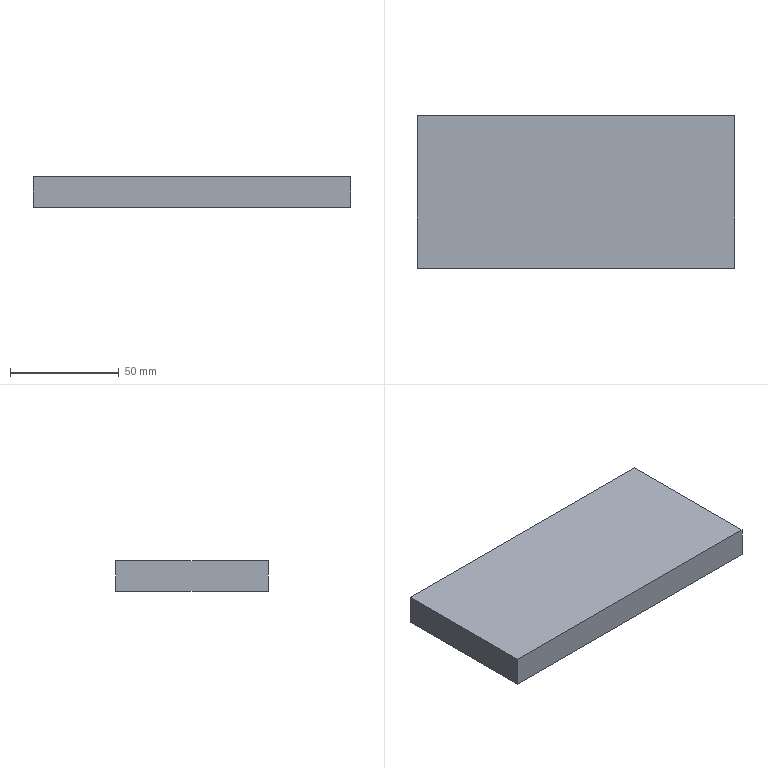Part | SolidWorks | features BaseBody 1 | 1 solid | 6 faces | box 146 x 70 x 14 mm | volume 143080 mm3 | plane 6
STEP:
#1=CARTESIAN_POINT('',(73.,-35.,-7.));
#2=VERTEX_POINT('',#1);
#3=CARTESIAN_POINT('',(73.,35.,-7.));
#4=VERTEX_POINT('',#3);
#5=CARTESIAN_POINT('',(73.,35.,-7.));
#6=DIRECTION('',(0.,1.,0.));
#7=VECTOR('',#6,1000.);
#8=LINE('',#5,#7);
#9=EDGE_CURVE('',#2,#4,#8,.T.);
#10=ORIENTED_EDGE('',*,*,#9,.T.);
#11=CARTESIAN_POINT('',(73.,35.,7.));
#12=VERTEX_POINT('',#11);
#13=CARTESIAN_POINT('',(73.,35.,7.));
#14=DIRECTION('',(0.,0.,-1.));
#15=VECTOR('',#14,1000.);
#16=LINE('',#13,#15);
#17=EDGE_CURVE('',#12,#4,#16,.T.);
#18=ORIENTED_EDGE('',*,*,#17,.F.);
#19=CARTESIAN_POINT('',(73.,-35.,7.));
#20=VERTEX_POINT('',#19);
#21=CARTESIAN_POINT('',(73.,35.,7.));
#22=DIRECTION('',(0.,1.,0.));
#23=VECTOR('',#22,1000.);
#24=LINE('',#21,#23);
#25=EDGE_CURVE('',#20,#12,#24,.T.);
#26=ORIENTED_EDGE('',*,*,#25,.F.);
#27=CARTESIAN_POINT('',(73.,-35.,7.));
#28=DIRECTION('',(0.,0.,-1.));
#29=VECTOR('',#28,1000.);
#30=LINE('',#27,#29);
#31=EDGE_CURVE('',#20,#2,#30,.T.);
#32=ORIENTED_EDGE('',*,*,#31,.T.);
#33=EDGE_LOOP('',(#10,#18,#26,#32));
#34=FACE_OUTER_BOUND('',#33,.T.);
#35=CARTESIAN_POINT('',(73.,35.,7.));
#36=DIRECTION('',(-1.,0.,0.));
#37=DIRECTION('',(0.,0.,1.));
#38=AXIS2_PLACEMENT_3D('',#35,#36,#37);
#39=PLANE('',#38);
#40=ADVANCED_FACE('',(#34),#39,.F.);
#41=CARTESIAN_POINT('',(-73.,35.,-7.));
#42=VERTEX_POINT('',#41);
#43=CARTESIAN_POINT('',(-73.,35.,-7.));
#44=DIRECTION('',(-1.,0.,0.));
#45=VECTOR('',#44,1000.);
#46=LINE('',#43,#45);
#47=EDGE_CURVE('',#4,#42,#46,.T.);
#48=ORIENTED_EDGE('',*,*,#47,.T.);
#49=CARTESIAN_POINT('',(-73.,35.,7.));
#50=VERTEX_POINT('',#49);
#51=CARTESIAN_POINT('',(-73.,35.,7.));
#52=DIRECTION('',(0.,0.,-1.));
#53=VECTOR('',#52,1000.);
#54=LINE('',#51,#53);
#55=EDGE_CURVE('',#50,#42,#54,.T.);
#56=ORIENTED_EDGE('',*,*,#55,.F.);
#57=CARTESIAN_POINT('',(-73.,35.,7.));
#58=DIRECTION('',(-1.,0.,0.));
#59=VECTOR('',#58,1000.);
#60=LINE('',#57,#59);
#61=EDGE_CURVE('',#12,#50,#60,.T.);
#62=ORIENTED_EDGE('',*,*,#61,.F.);
#63=ORIENTED_EDGE('',*,*,#17,.T.);
#64=EDGE_LOOP('',(#48,#56,#62,#63));
#65=FACE_OUTER_BOUND('',#64,.T.);
#66=CARTESIAN_POINT('',(-73.,35.,7.));
#67=DIRECTION('',(0.,-1.,0.));
#68=DIRECTION('',(0.,0.,-1.));
#69=AXIS2_PLACEMENT_3D('',#66,#67,#68);
#70=PLANE('',#69);
#71=ADVANCED_FACE('',(#65),#70,.F.);
#72=CARTESIAN_POINT('',(-73.,-35.,-7.));
#73=VERTEX_POINT('',#72);
#74=CARTESIAN_POINT('',(-73.,35.,-7.));
#75=DIRECTION('',(0.,-1.,0.));
#76=VECTOR('',#75,1000.);
#77=LINE('',#74,#76);
#78=EDGE_CURVE('',#42,#73,#77,.T.);
#79=ORIENTED_EDGE('',*,*,#78,.T.);
#80=CARTESIAN_POINT('',(-73.,-35.,7.));
#81=VERTEX_POINT('',#80);
#82=CARTESIAN_POINT('',(-73.,-35.,7.));
#83=DIRECTION('',(0.,0.,-1.));
#84=VECTOR('',#83,1000.);
#85=LINE('',#82,#84);
#86=EDGE_CURVE('',#81,#73,#85,.T.);
#87=ORIENTED_EDGE('',*,*,#86,.F.);
#88=CARTESIAN_POINT('',(-73.,35.,7.));
#89=DIRECTION('',(0.,-1.,0.));
#90=VECTOR('',#89,1000.);
#91=LINE('',#88,#90);
#92=EDGE_CURVE('',#50,#81,#91,.T.);
#93=ORIENTED_EDGE('',*,*,#92,.F.);
#94=ORIENTED_EDGE('',*,*,#55,.T.);
#95=EDGE_LOOP('',(#79,#87,#93,#94));
#96=FACE_OUTER_BOUND('',#95,.T.);
#97=CARTESIAN_POINT('',(-73.,35.,7.));
#98=DIRECTION('',(1.,0.,0.));
#99=DIRECTION('',(0.,0.,-1.));
#100=AXIS2_PLACEMENT_3D('',#97,#98,#99);
#101=PLANE('',#100);
#102=ADVANCED_FACE('',(#96),#101,.F.);
#103=CARTESIAN_POINT('',(-73.,-35.,-7.));
#104=DIRECTION('',(1.,0.,0.));
#105=VECTOR('',#104,1000.);
#106=LINE('',#103,#105);
#107=EDGE_CURVE('',#73,#2,#106,.T.);
#108=ORIENTED_EDGE('',*,*,#107,.T.);
#109=ORIENTED_EDGE('',*,*,#31,.F.);
#110=CARTESIAN_POINT('',(-73.,-35.,7.));
#111=DIRECTION('',(1.,0.,0.));
#112=VECTOR('',#111,1000.);
#113=LINE('',#110,#112);
#114=EDGE_CURVE('',#81,#20,#113,.T.);
#115=ORIENTED_EDGE('',*,*,#114,.F.);
#116=ORIENTED_EDGE('',*,*,#86,.T.);
#117=EDGE_LOOP('',(#108,#109,#115,#116));
#118=FACE_OUTER_BOUND('',#117,.T.);
#119=CARTESIAN_POINT('',(-73.,-35.,7.));
#120=DIRECTION('',(0.,1.,0.));
#121=DIRECTION('',(0.,0.,1.));
#122=AXIS2_PLACEMENT_3D('',#119,#120,#121);
#123=PLANE('',#122);
#124=ADVANCED_FACE('',(#118),#123,.F.);
#125=ORIENTED_EDGE('',*,*,#25,.T.);
#126=ORIENTED_EDGE('',*,*,#61,.T.);
#127=ORIENTED_EDGE('',*,*,#92,.T.);
#128=ORIENTED_EDGE('',*,*,#114,.T.);
#129=EDGE_LOOP('',(#125,#126,#127,#128));
#130=FACE_OUTER_BOUND('',#129,.T.);
#131=CARTESIAN_POINT('',(0.,0.,7.));
#132=DIRECTION('',(0.,0.,1.));
#133=DIRECTION('',(1.,0.,0.));
#134=AXIS2_PLACEMENT_3D('',#131,#132,#133);
#135=PLANE('',#134);
#136=ADVANCED_FACE('',(#130),#135,.T.);
#137=ORIENTED_EDGE('',*,*,#9,.F.);
#138=ORIENTED_EDGE('',*,*,#107,.F.);
#139=ORIENTED_EDGE('',*,*,#78,.F.);
#140=ORIENTED_EDGE('',*,*,#47,.F.);
#141=EDGE_LOOP('',(#137,#138,#139,#140));
#142=FACE_OUTER_BOUND('',#141,.T.);
#143=CARTESIAN_POINT('',(0.,0.,-7.));
#144=DIRECTION('',(0.,0.,1.));
#145=DIRECTION('',(1.,0.,0.));
#146=AXIS2_PLACEMENT_3D('',#143,#144,#145);
#147=PLANE('',#146);
#148=ADVANCED_FACE('',(#142),#147,.F.);
#149=CLOSED_SHELL('',(#40,#71,#102,#124,#136,#148));
#150=MANIFOLD_SOLID_BREP('',#149);
#151=CARTESIAN_POINT('',(0.,0.,0.));
#152=DIRECTION('',(0.,0.,1.));
#153=DIRECTION('',(1.,0.,0.));
#154=AXIS2_PLACEMENT_3D('',#151,#152,#153);
#155=(LENGTH_UNIT()NAMED_UNIT(*)SI_UNIT(.MILLI.,.METRE.));
#156=UNCERTAINTY_MEASURE_WITH_UNIT(LENGTH_MEASURE(0.00001),#155,'','');
#157=(NAMED_UNIT(*)PLANE_ANGLE_UNIT()SI_UNIT($,.RADIAN.));
#158=(NAMED_UNIT(*)SI_UNIT($,.STERADIAN.)SOLID_ANGLE_UNIT());
#159=(GEOMETRIC_REPRESENTATION_CONTEXT(3)GLOBAL_UNCERTAINTY_ASSIGNED_CONTEXT((#156))GLOBAL_UNIT_ASSIGNED_CONTEXT((#155,#157,#158))REPRESENTATION_CONTEXT('',''));
#160=ADVANCED_BREP_SHAPE_REPRESENTATION('',(#150,#154),#159);